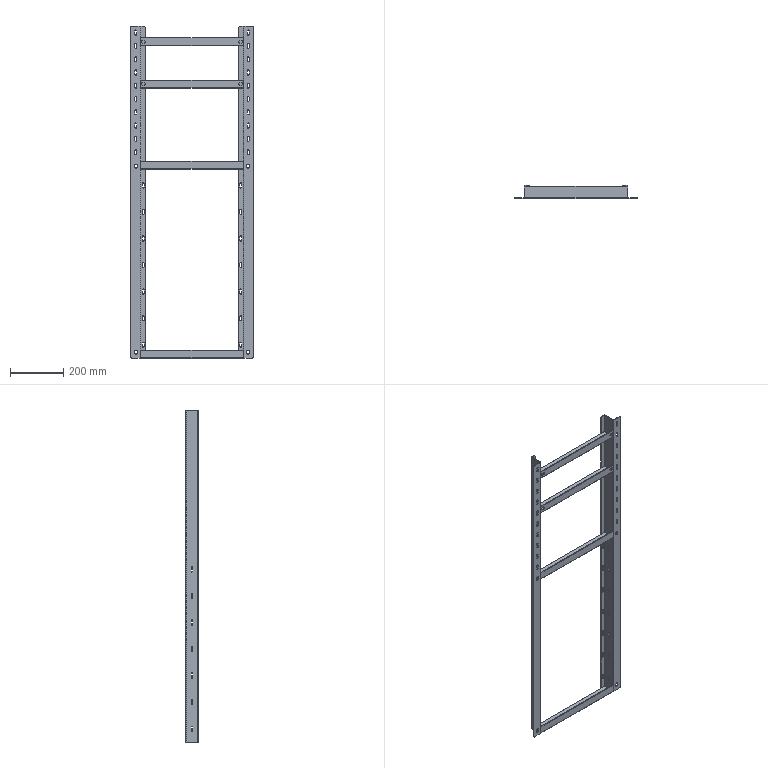Part | SolidWorks | 6 solids | 362 faces | box 463 x 50 x 1250 mm | volume 955457 mm3 | plane 204 | cylinder 158 | commonest cylinder face diameters 7 x118 10 x16 0.2 x8 12 x8 4.2 x4 6.2 x4